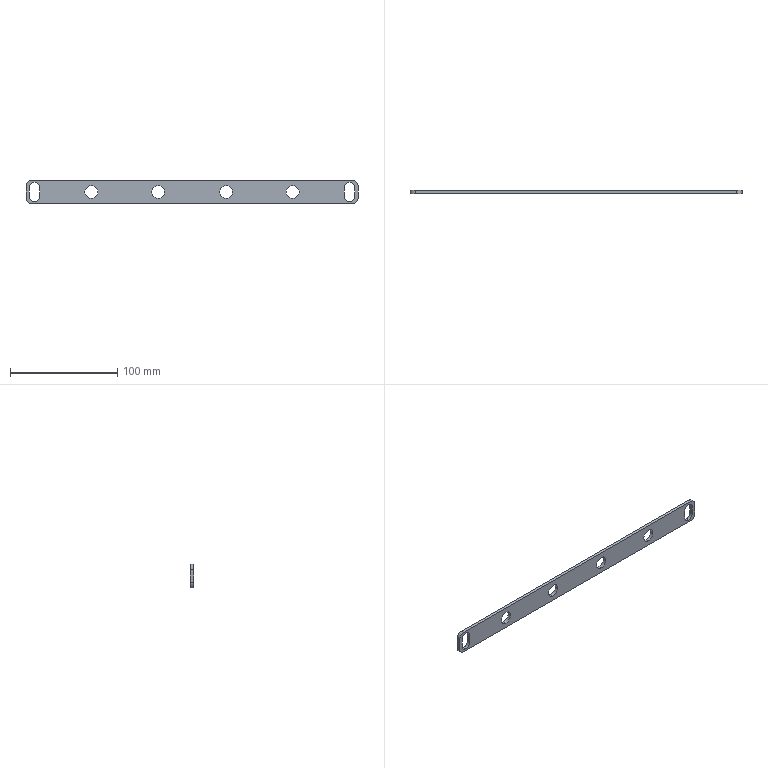Part | 1 solid | 28 faces | box 310 x 3 x 22 mm | volume 18087 mm3 | cylinder 18 | plane 10 | commonest cylinder face diameters 10 x10 12 x8
STEP:
#1=CARTESIAN_POINT('',(152.,3.,-4.));
#2=VERTEX_POINT('',#1);
#3=CARTESIAN_POINT('',(147.,3.,-9.));
#4=VERTEX_POINT('',#3);
#5=CARTESIAN_POINT('',(147.,3.,-4.));
#6=DIRECTION('',(0.,1.,0.));
#7=DIRECTION('',(0.,0.,-1.));
#8=AXIS2_PLACEMENT_3D('',#5,#6,#7);
#9=CIRCLE('',#8,5.);
#10=EDGE_CURVE('',#2,#4,#9,.T.);
#11=ORIENTED_EDGE('',*,*,#10,.T.);
#12=CARTESIAN_POINT('',(147.,0.,-9.));
#13=VERTEX_POINT('',#12);
#14=CARTESIAN_POINT('',(147.,3.,-9.));
#15=DIRECTION('',(0.,-1.,0.));
#16=VECTOR('',#15,1000.);
#17=LINE('',#14,#16);
#18=EDGE_CURVE('',#4,#13,#17,.T.);
#19=ORIENTED_EDGE('',*,*,#18,.T.);
#20=CARTESIAN_POINT('',(152.,0.,-4.));
#21=VERTEX_POINT('',#20);
#22=CARTESIAN_POINT('',(147.,0.,-4.));
#23=DIRECTION('',(0.,1.,0.));
#24=DIRECTION('',(0.,0.,-1.));
#25=AXIS2_PLACEMENT_3D('',#22,#23,#24);
#26=CIRCLE('',#25,5.);
#27=EDGE_CURVE('',#21,#13,#26,.T.);
#28=ORIENTED_EDGE('',*,*,#27,.F.);
#29=CARTESIAN_POINT('',(152.,3.,-4.));
#30=DIRECTION('',(0.,-1.,0.));
#31=VECTOR('',#30,1000.);
#32=LINE('',#29,#31);
#33=EDGE_CURVE('',#2,#21,#32,.T.);
#34=ORIENTED_EDGE('',*,*,#33,.F.);
#35=EDGE_LOOP('',(#11,#19,#28,#34));
#36=FACE_OUTER_BOUND('',#35,.T.);
#37=CARTESIAN_POINT('',(147.,3.,-4.));
#38=DIRECTION('',(0.,-1.,0.));
#39=DIRECTION('',(0.,0.,-1.));
#40=AXIS2_PLACEMENT_3D('',#37,#38,#39);
#41=CYLINDRICAL_SURFACE('',#40,5.);
#42=ADVANCED_FACE('',(#36),#41,.F.);
#43=CARTESIAN_POINT('',(94.,3.,-6.));
#44=VERTEX_POINT('',#43);
#45=CARTESIAN_POINT('',(94.,3.,6.));
#46=VERTEX_POINT('',#45);
#47=CARTESIAN_POINT('',(94.,3.,0.));
#48=DIRECTION('',(0.,1.,0.));
#49=DIRECTION('',(0.,0.,1.));
#50=AXIS2_PLACEMENT_3D('',#47,#48,#49);
#51=CIRCLE('',#50,6.);
#52=EDGE_CURVE('',#44,#46,#51,.T.);
#53=ORIENTED_EDGE('',*,*,#52,.T.);
#54=CARTESIAN_POINT('',(94.,0.,6.));
#55=VERTEX_POINT('',#54);
#56=CARTESIAN_POINT('',(94.,3.,6.));
#57=DIRECTION('',(0.,-1.,0.));
#58=VECTOR('',#57,1000.);
#59=LINE('',#56,#58);
#60=EDGE_CURVE('',#46,#55,#59,.T.);
#61=ORIENTED_EDGE('',*,*,#60,.T.);
#62=CARTESIAN_POINT('',(94.,0.,-6.));
#63=VERTEX_POINT('',#62);
#64=CARTESIAN_POINT('',(94.,0.,0.));
#65=DIRECTION('',(0.,1.,0.));
#66=DIRECTION('',(0.,0.,1.));
#67=AXIS2_PLACEMENT_3D('',#64,#65,#66);
#68=CIRCLE('',#67,6.);
#69=EDGE_CURVE('',#63,#55,#68,.T.);
#70=ORIENTED_EDGE('',*,*,#69,.F.);
#71=CARTESIAN_POINT('',(94.,3.,-6.));
#72=DIRECTION('',(0.,-1.,0.));
#73=VECTOR('',#72,1000.);
#74=LINE('',#71,#73);
#75=EDGE_CURVE('',#44,#63,#74,.T.);
#76=ORIENTED_EDGE('',*,*,#75,.F.);
#77=EDGE_LOOP('',(#53,#61,#70,#76));
#78=FACE_OUTER_BOUND('',#77,.T.);
#79=CARTESIAN_POINT('',(94.,3.,0.));
#80=DIRECTION('',(0.,-1.,0.));
#81=DIRECTION('',(0.,0.,-1.));
#82=AXIS2_PLACEMENT_3D('',#79,#80,#81);
#83=CYLINDRICAL_SURFACE('',#82,6.);
#84=ADVANCED_FACE('',(#78),#83,.F.);
#85=CARTESIAN_POINT('',(31.8,3.,-6.));
#86=VERTEX_POINT('',#85);
#87=CARTESIAN_POINT('',(31.8,3.,6.));
#88=VERTEX_POINT('',#87);
#89=CARTESIAN_POINT('',(31.8,3.,0.));
#90=DIRECTION('',(0.,1.,0.));
#91=DIRECTION('',(0.,0.,1.));
#92=AXIS2_PLACEMENT_3D('',#89,#90,#91);
#93=CIRCLE('',#92,6.);
#94=EDGE_CURVE('',#86,#88,#93,.T.);
#95=ORIENTED_EDGE('',*,*,#94,.T.);
#96=CARTESIAN_POINT('',(31.8,0.,6.));
#97=VERTEX_POINT('',#96);
#98=CARTESIAN_POINT('',(31.8,3.,6.));
#99=DIRECTION('',(0.,-1.,0.));
#100=VECTOR('',#99,1000.);
#101=LINE('',#98,#100);
#102=EDGE_CURVE('',#88,#97,#101,.T.);
#103=ORIENTED_EDGE('',*,*,#102,.T.);
#104=CARTESIAN_POINT('',(31.8,0.,-6.));
#105=VERTEX_POINT('',#104);
#106=CARTESIAN_POINT('',(31.8,0.,0.));
#107=DIRECTION('',(0.,1.,0.));
#108=DIRECTION('',(0.,0.,1.));
#109=AXIS2_PLACEMENT_3D('',#106,#107,#108);
#110=CIRCLE('',#109,6.);
#111=EDGE_CURVE('',#105,#97,#110,.T.);
#112=ORIENTED_EDGE('',*,*,#111,.F.);
#113=CARTESIAN_POINT('',(31.8,3.,-6.));
#114=DIRECTION('',(0.,-1.,0.));
#115=VECTOR('',#114,1000.);
#116=LINE('',#113,#115);
#117=EDGE_CURVE('',#86,#105,#116,.T.);
#118=ORIENTED_EDGE('',*,*,#117,.F.);
#119=EDGE_LOOP('',(#95,#103,#112,#118));
#120=FACE_OUTER_BOUND('',#119,.T.);
#121=CARTESIAN_POINT('',(31.8,3.,0.));
#122=DIRECTION('',(0.,-1.,0.));
#123=DIRECTION('',(0.,0.,-1.));
#124=AXIS2_PLACEMENT_3D('',#121,#122,#123);
#125=CYLINDRICAL_SURFACE('',#124,6.);
#126=ADVANCED_FACE('',(#120),#125,.F.);
#127=CARTESIAN_POINT('',(-31.7,3.,-6.));
#128=VERTEX_POINT('',#127);
#129=CARTESIAN_POINT('',(-31.7,3.,6.));
#130=VERTEX_POINT('',#129);
#131=CARTESIAN_POINT('',(-31.7,3.,0.));
#132=DIRECTION('',(0.,1.,0.));
#133=DIRECTION('',(0.,0.,1.));
#134=AXIS2_PLACEMENT_3D('',#131,#132,#133);
#135=CIRCLE('',#134,6.);
#136=EDGE_CURVE('',#128,#130,#135,.T.);
#137=ORIENTED_EDGE('',*,*,#136,.T.);
#138=CARTESIAN_POINT('',(-31.7,0.,6.));
#139=VERTEX_POINT('',#138);
#140=CARTESIAN_POINT('',(-31.7,3.,6.));
#141=DIRECTION('',(0.,-1.,0.));
#142=VECTOR('',#141,1000.);
#143=LINE('',#140,#142);
#144=EDGE_CURVE('',#130,#139,#143,.T.);
#145=ORIENTED_EDGE('',*,*,#144,.T.);
#146=CARTESIAN_POINT('',(-31.7,0.,-6.));
#147=VERTEX_POINT('',#146);
#148=CARTESIAN_POINT('',(-31.7,0.,0.));
#149=DIRECTION('',(0.,1.,0.));
#150=DIRECTION('',(0.,0.,1.));
#151=AXIS2_PLACEMENT_3D('',#148,#149,#150);
#152=CIRCLE('',#151,6.);
#153=EDGE_CURVE('',#147,#139,#152,.T.);
#154=ORIENTED_EDGE('',*,*,#153,.F.);
#155=CARTESIAN_POINT('',(-31.7,3.,-6.));
#156=DIRECTION('',(0.,-1.,0.));
#157=VECTOR('',#156,1000.);
#158=LINE('',#155,#157);
#159=EDGE_CURVE('',#128,#147,#158,.T.);
#160=ORIENTED_EDGE('',*,*,#159,.F.);
#161=EDGE_LOOP('',(#137,#145,#154,#160));
#162=FACE_OUTER_BOUND('',#161,.T.);
#163=CARTESIAN_POINT('',(-31.7,3.,0.));
#164=DIRECTION('',(0.,-1.,0.));
#165=DIRECTION('',(0.,0.,-1.));
#166=AXIS2_PLACEMENT_3D('',#163,#164,#165);
#167=CYLINDRICAL_SURFACE('',#166,6.);
#168=ADVANCED_FACE('',(#162),#167,.F.);
#169=CARTESIAN_POINT('',(-94.,3.,-6.));
#170=VERTEX_POINT('',#169);
#171=CARTESIAN_POINT('',(-94.,3.,6.));
#172=VERTEX_POINT('',#171);
#173=CARTESIAN_POINT('',(-94.,3.,0.));
#174=DIRECTION('',(0.,1.,0.));
#175=DIRECTION('',(0.,0.,1.));
#176=AXIS2_PLACEMENT_3D('',#173,#174,#175);
#177=CIRCLE('',#176,6.);
#178=EDGE_CURVE('',#170,#172,#177,.T.);
#179=ORIENTED_EDGE('',*,*,#178,.T.);
#180=CARTESIAN_POINT('',(-94.,0.,6.));
#181=VERTEX_POINT('',#180);
#182=CARTESIAN_POINT('',(-94.,3.,6.));
#183=DIRECTION('',(0.,-1.,0.));
#184=VECTOR('',#183,1000.);
#185=LINE('',#182,#184);
#186=EDGE_CURVE('',#172,#181,#185,.T.);
#187=ORIENTED_EDGE('',*,*,#186,.T.);
#188=CARTESIAN_POINT('',(-94.,0.,-6.));
#189=VERTEX_POINT('',#188);
#190=CARTESIAN_POINT('',(-94.,0.,0.));
#191=DIRECTION('',(0.,1.,0.));
#192=DIRECTION('',(0.,0.,1.));
#193=AXIS2_PLACEMENT_3D('',#190,#191,#192);
#194=CIRCLE('',#193,6.);
#195=EDGE_CURVE('',#189,#181,#194,.T.);
#196=ORIENTED_EDGE('',*,*,#195,.F.);
#197=CARTESIAN_POINT('',(-94.,3.,-6.));
#198=DIRECTION('',(0.,-1.,0.));
#199=VECTOR('',#198,1000.);
#200=LINE('',#197,#199);
#201=EDGE_CURVE('',#170,#189,#200,.T.);
#202=ORIENTED_EDGE('',*,*,#201,.F.);
#203=EDGE_LOOP('',(#179,#187,#196,#202));
#204=FACE_OUTER_BOUND('',#203,.T.);
#205=CARTESIAN_POINT('',(-94.,3.,0.));
#206=DIRECTION('',(0.,-1.,0.));
#207=DIRECTION('',(0.,0.,-1.));
#208=AXIS2_PLACEMENT_3D('',#205,#206,#207);
#209=CYLINDRICAL_SURFACE('',#208,6.);
#210=ADVANCED_FACE('',(#204),#209,.F.);
#211=CARTESIAN_POINT('',(-142.,3.,-4.));
#212=VERTEX_POINT('',#211);
#213=CARTESIAN_POINT('',(-147.,3.,-9.));
#214=VERTEX_POINT('',#213);
#215=CARTESIAN_POINT('',(-147.,3.,-4.));
#216=DIRECTION('',(0.,1.,0.));
#217=DIRECTION('',(0.,0.,1.));
#218=AXIS2_PLACEMENT_3D('',#215,#216,#217);
#219=CIRCLE('',#218,5.);
#220=EDGE_CURVE('',#212,#214,#219,.T.);
#221=ORIENTED_EDGE('',*,*,#220,.T.);
#222=CARTESIAN_POINT('',(-147.,0.,-9.));
#223=VERTEX_POINT('',#222);
#224=CARTESIAN_POINT('',(-147.,3.,-9.));
#225=DIRECTION('',(0.,-1.,0.));
#226=VECTOR('',#225,1000.);
#227=LINE('',#224,#226);
#228=EDGE_CURVE('',#214,#223,#227,.T.);
#229=ORIENTED_EDGE('',*,*,#228,.T.);
#230=CARTESIAN_POINT('',(-142.,0.,-4.));
#231=VERTEX_POINT('',#230);
#232=CARTESIAN_POINT('',(-147.,0.,-4.));
#233=DIRECTION('',(0.,1.,0.));
#234=DIRECTION('',(0.,0.,1.));
#235=AXIS2_PLACEMENT_3D('',#232,#233,#234);
#236=CIRCLE('',#235,5.);
#237=EDGE_CURVE('',#231,#223,#236,.T.);
#238=ORIENTED_EDGE('',*,*,#237,.F.);
#239=CARTESIAN_POINT('',(-142.,3.,-4.));
#240=DIRECTION('',(0.,-1.,0.));
#241=VECTOR('',#240,1000.);
#242=LINE('',#239,#241);
#243=EDGE_CURVE('',#212,#231,#242,.T.);
#244=ORIENTED_EDGE('',*,*,#243,.F.);
#245=EDGE_LOOP('',(#221,#229,#238,#244));
#246=FACE_OUTER_BOUND('',#245,.T.);
#247=CARTESIAN_POINT('',(-147.,3.,-4.));
#248=DIRECTION('',(0.,-1.,0.));
#249=DIRECTION('',(0.,0.,-1.));
#250=AXIS2_PLACEMENT_3D('',#247,#248,#249);
#251=CYLINDRICAL_SURFACE('',#250,5.);
#252=ADVANCED_FACE('',(#246),#251,.F.);
#253=ORIENTED_EDGE('',*,*,#94,.F.);
#254=CARTESIAN_POINT('',(31.8,3.,0.));
#255=DIRECTION('',(0.,1.,0.));
#256=DIRECTION('',(0.,0.,1.));
#257=AXIS2_PLACEMENT_3D('',#254,#255,#256);
#258=CIRCLE('',#257,6.);
#259=EDGE_CURVE('',#88,#86,#258,.T.);
#260=ORIENTED_EDGE('',*,*,#259,.F.);
#261=EDGE_LOOP('',(#253,#260));
#262=FACE_BOUND('',#261,.T.);
#263=ORIENTED_EDGE('',*,*,#178,.F.);
#264=CARTESIAN_POINT('',(-94.,3.,0.));
#265=DIRECTION('',(0.,1.,0.));
#266=DIRECTION('',(0.,0.,1.));
#267=AXIS2_PLACEMENT_3D('',#264,#265,#266);
#268=CIRCLE('',#267,6.);
#269=EDGE_CURVE('',#172,#170,#268,.T.);
#270=ORIENTED_EDGE('',*,*,#269,.F.);
#271=EDGE_LOOP('',(#263,#270));
#272=FACE_BOUND('',#271,.T.);
#273=CARTESIAN_POINT('',(-150.,3.,11.));
#274=VERTEX_POINT('',#273);
#275=CARTESIAN_POINT('',(150.,3.,11.));
#276=VERTEX_POINT('',#275);
#277=CARTESIAN_POINT('',(-155.,3.,11.));
#278=DIRECTION('',(1.,0.,0.));
#279=VECTOR('',#278,1000.);
#280=LINE('',#277,#279);
#281=EDGE_CURVE('',#274,#276,#280,.T.);
#282=ORIENTED_EDGE('',*,*,#281,.T.);
#283=CARTESIAN_POINT('',(155.,3.,6.));
#284=VERTEX_POINT('',#283);
#285=CARTESIAN_POINT('',(150.,3.,6.));
#286=DIRECTION('',(0.,1.,0.));
#287=DIRECTION('',(0.,0.,1.));
#288=AXIS2_PLACEMENT_3D('',#285,#286,#287);
#289=CIRCLE('',#288,5.);
#290=EDGE_CURVE('',#276,#284,#289,.T.);
#291=ORIENTED_EDGE('',*,*,#290,.T.);
#292=CARTESIAN_POINT('',(155.,3.,-6.));
#293=VERTEX_POINT('',#292);
#294=CARTESIAN_POINT('',(155.,3.,-11.));
#295=DIRECTION('',(0.,0.,-1.));
#296=VECTOR('',#295,1000.);
#297=LINE('',#294,#296);
#298=EDGE_CURVE('',#284,#293,#297,.T.);
#299=ORIENTED_EDGE('',*,*,#298,.T.);
#300=CARTESIAN_POINT('',(150.,3.,-11.));
#301=VERTEX_POINT('',#300);
#302=CARTESIAN_POINT('',(150.,3.,-6.));
#303=DIRECTION('',(0.,1.,0.));
#304=DIRECTION('',(0.,0.,1.));
#305=AXIS2_PLACEMENT_3D('',#302,#303,#304);
#306=CIRCLE('',#305,5.);
#307=EDGE_CURVE('',#293,#301,#306,.T.);
#308=ORIENTED_EDGE('',*,*,#307,.T.);
#309=CARTESIAN_POINT('',(-150.,3.,-11.));
#310=VERTEX_POINT('',#309);
#311=CARTESIAN_POINT('',(-155.,3.,-11.));
#312=DIRECTION('',(-1.,0.,0.));
#313=VECTOR('',#312,1000.);
#314=LINE('',#311,#313);
#315=EDGE_CURVE('',#301,#310,#314,.T.);
#316=ORIENTED_EDGE('',*,*,#315,.T.);
#317=CARTESIAN_POINT('',(-155.,3.,-6.));
#318=VERTEX_POINT('',#317);
#319=CARTESIAN_POINT('',(-150.,3.,-6.));
#320=DIRECTION('',(0.,1.,0.));
#321=DIRECTION('',(0.,0.,1.));
#322=AXIS2_PLACEMENT_3D('',#319,#320,#321);
#323=CIRCLE('',#322,5.);
#324=EDGE_CURVE('',#310,#318,#323,.T.);
#325=ORIENTED_EDGE('',*,*,#324,.T.);
#326=CARTESIAN_POINT('',(-155.,3.,6.));
#327=VERTEX_POINT('',#326);
#328=CARTESIAN_POINT('',(-155.,3.,-11.));
#329=DIRECTION('',(0.,0.,1.));
#330=VECTOR('',#329,1000.);
#331=LINE('',#328,#330);
#332=EDGE_CURVE('',#318,#327,#331,.T.);
#333=ORIENTED_EDGE('',*,*,#332,.T.);
#334=CARTESIAN_POINT('',(-150.,3.,6.));
#335=DIRECTION('',(0.,1.,0.));
#336=DIRECTION('',(0.,0.,1.));
#337=AXIS2_PLACEMENT_3D('',#334,#335,#336);
#338=CIRCLE('',#337,5.);
#339=EDGE_CURVE('',#327,#274,#338,.T.);
#340=ORIENTED_EDGE('',*,*,#339,.T.);
#341=EDGE_LOOP('',(#282,#291,#299,#308,#316,#325,#333,#340));
#342=FACE_OUTER_BOUND('',#341,.T.);
#343=CARTESIAN_POINT('',(-142.,3.,4.));
#344=VERTEX_POINT('',#343);
#345=CARTESIAN_POINT('',(-142.,3.,4.));
#346=DIRECTION('',(0.,0.,-1.));
#347=VECTOR('',#346,1000.);
#348=LINE('',#345,#347);
#349=EDGE_CURVE('',#344,#212,#348,.T.);
#350=ORIENTED_EDGE('',*,*,#349,.F.);
#351=CARTESIAN_POINT('',(-152.,3.,4.));
#352=VERTEX_POINT('',#351);
#353=CARTESIAN_POINT('',(-147.,3.,4.));
#354=DIRECTION('',(0.,1.,0.));
#355=DIRECTION('',(0.,0.,1.));
#356=AXIS2_PLACEMENT_3D('',#353,#354,#355);
#357=CIRCLE('',#356,5.);
#358=EDGE_CURVE('',#352,#344,#357,.T.);
#359=ORIENTED_EDGE('',*,*,#358,.F.);
#360=CARTESIAN_POINT('',(-152.,3.,-4.));
#361=VERTEX_POINT('',#360);
#362=CARTESIAN_POINT('',(-152.,3.,4.));
#363=DIRECTION('',(0.,0.,1.));
#364=VECTOR('',#363,1000.);
#365=LINE('',#362,#364);
#366=EDGE_CURVE('',#361,#352,#365,.T.);
#367=ORIENTED_EDGE('',*,*,#366,.F.);
#368=CARTESIAN_POINT('',(-147.,3.,-4.));
#369=DIRECTION('',(0.,1.,0.));
#370=DIRECTION('',(0.,0.,1.));
#371=AXIS2_PLACEMENT_3D('',#368,#369,#370);
#372=CIRCLE('',#371,5.);
#373=EDGE_CURVE('',#214,#361,#372,.T.);
#374=ORIENTED_EDGE('',*,*,#373,.F.);
#375=ORIENTED_EDGE('',*,*,#220,.F.);
#376=EDGE_LOOP('',(#350,#359,#367,#374,#375));
#377=FACE_BOUND('',#376,.T.);
#378=ORIENTED_EDGE('',*,*,#136,.F.);
#379=CARTESIAN_POINT('',(-31.7,3.,0.));
#380=DIRECTION('',(0.,1.,0.));
#381=DIRECTION('',(0.,0.,1.));
#382=AXIS2_PLACEMENT_3D('',#379,#380,#381);
#383=CIRCLE('',#382,6.);
#384=EDGE_CURVE('',#130,#128,#383,.T.);
#385=ORIENTED_EDGE('',*,*,#384,.F.);
#386=EDGE_LOOP('',(#378,#385));
#387=FACE_BOUND('',#386,.T.);
#388=ORIENTED_EDGE('',*,*,#52,.F.);
#389=CARTESIAN_POINT('',(94.,3.,0.));
#390=DIRECTION('',(0.,1.,0.));
#391=DIRECTION('',(0.,0.,1.));
#392=AXIS2_PLACEMENT_3D('',#389,#390,#391);
#393=CIRCLE('',#392,6.);
#394=EDGE_CURVE('',#46,#44,#393,.T.);
#395=ORIENTED_EDGE('',*,*,#394,.F.);
#396=EDGE_LOOP('',(#388,#395));
#397=FACE_BOUND('',#396,.T.);
#398=CARTESIAN_POINT('',(152.,3.,4.));
#399=VERTEX_POINT('',#398);
#400=CARTESIAN_POINT('',(152.,3.,4.));
#401=DIRECTION('',(0.,0.,-1.));
#402=VECTOR('',#401,1000.);
#403=LINE('',#400,#402);
#404=EDGE_CURVE('',#399,#2,#403,.T.);
#405=ORIENTED_EDGE('',*,*,#404,.F.);
#406=CARTESIAN_POINT('',(142.,3.,4.));
#407=VERTEX_POINT('',#406);
#408=CARTESIAN_POINT('',(147.,3.,4.));
#409=DIRECTION('',(0.,1.,0.));
#410=DIRECTION('',(0.,0.,-1.));
#411=AXIS2_PLACEMENT_3D('',#408,#409,#410);
#412=CIRCLE('',#411,5.);
#413=EDGE_CURVE('',#407,#399,#412,.T.);
#414=ORIENTED_EDGE('',*,*,#413,.F.);
#415=CARTESIAN_POINT('',(142.,3.,-4.));
#416=VERTEX_POINT('',#415);
#417=CARTESIAN_POINT('',(142.,3.,4.));
#418=DIRECTION('',(0.,0.,1.));
#419=VECTOR('',#418,1000.);
#420=LINE('',#417,#419);
#421=EDGE_CURVE('',#416,#407,#420,.T.);
#422=ORIENTED_EDGE('',*,*,#421,.F.);
#423=CARTESIAN_POINT('',(147.,3.,-4.));
#424=DIRECTION('',(0.,1.,0.));
#425=DIRECTION('',(0.,0.,-1.));
#426=AXIS2_PLACEMENT_3D('',#423,#424,#425);
#427=CIRCLE('',#426,5.);
#428=EDGE_CURVE('',#4,#416,#427,.T.);
#429=ORIENTED_EDGE('',*,*,#428,.F.);
#430=ORIENTED_EDGE('',*,*,#10,.F.);
#431=EDGE_LOOP('',(#405,#414,#422,#429,#430));
#432=FACE_BOUND('',#431,.T.);
#433=CARTESIAN_POINT('',(0.,3.,0.));
#434=DIRECTION('',(0.,1.,0.));
#435=DIRECTION('',(0.,0.,1.));
#436=AXIS2_PLACEMENT_3D('',#433,#434,#435);
#437=PLANE('',#436);
#438=ADVANCED_FACE('',(#262,#272,#342,#377,#387,#397,#432),#437,.T.);
#439=ORIENTED_EDGE('',*,*,#69,.T.);
#440=CARTESIAN_POINT('',(94.,0.,0.));
#441=DIRECTION('',(0.,1.,0.));
#442=DIRECTION('',(0.,0.,1.));
#443=AXIS2_PLACEMENT_3D('',#440,#441,#442);
#444=CIRCLE('',#443,6.);
#445=EDGE_CURVE('',#55,#63,#444,.T.);
#446=ORIENTED_EDGE('',*,*,#445,.T.);
#447=EDGE_LOOP('',(#439,#446));
#448=FACE_BOUND('',#447,.T.);
#449=ORIENTED_EDGE('',*,*,#111,.T.);
#450=CARTESIAN_POINT('',(31.8,0.,0.));
#451=DIRECTION('',(0.,1.,0.));
#452=DIRECTION('',(0.,0.,1.));
#453=AXIS2_PLACEMENT_3D('',#450,#451,#452);
#454=CIRCLE('',#453,6.);
#455=EDGE_CURVE('',#97,#105,#454,.T.);
#456=ORIENTED_EDGE('',*,*,#455,.T.);
#457=EDGE_LOOP('',(#449,#456));
#458=FACE_BOUND('',#457,.T.);
#459=ORIENTED_EDGE('',*,*,#153,.T.);
#460=CARTESIAN_POINT('',(-31.7,0.,0.));
#461=DIRECTION('',(0.,1.,0.));
#462=DIRECTION('',(0.,0.,1.));
#463=AXIS2_PLACEMENT_3D('',#460,#461,#462);
#464=CIRCLE('',#463,6.);
#465=EDGE_CURVE('',#139,#147,#464,.T.);
#466=ORIENTED_EDGE('',*,*,#465,.T.);
#467=EDGE_LOOP('',(#459,#466));
#468=FACE_BOUND('',#467,.T.);
#469=ORIENTED_EDGE('',*,*,#195,.T.);
#470=CARTESIAN_POINT('',(-94.,0.,0.));
#471=DIRECTION('',(0.,1.,0.));
#472=DIRECTION('',(0.,0.,1.));
#473=AXIS2_PLACEMENT_3D('',#470,#471,#472);
#474=CIRCLE('',#473,6.);
#475=EDGE_CURVE('',#181,#189,#474,.T.);
#476=ORIENTED_EDGE('',*,*,#475,.T.);
#477=EDGE_LOOP('',(#469,#476));
#478=FACE_BOUND('',#477,.T.);
#479=CARTESIAN_POINT('',(-152.,0.,4.));
#480=VERTEX_POINT('',#479);
#481=CARTESIAN_POINT('',(-142.,0.,4.));
#482=VERTEX_POINT('',#481);
#483=CARTESIAN_POINT('',(-147.,0.,4.));
#484=DIRECTION('',(0.,1.,0.));
#485=DIRECTION('',(0.,0.,1.));
#486=AXIS2_PLACEMENT_3D('',#483,#484,#485);
#487=CIRCLE('',#486,5.);
#488=EDGE_CURVE('',#480,#482,#487,.T.);
#489=ORIENTED_EDGE('',*,*,#488,.T.);
#490=CARTESIAN_POINT('',(-142.,0.,4.));
#491=DIRECTION('',(0.,0.,-1.));
#492=VECTOR('',#491,1000.);
#493=LINE('',#490,#492);
#494=EDGE_CURVE('',#482,#231,#493,.T.);
#495=ORIENTED_EDGE('',*,*,#494,.T.);
#496=ORIENTED_EDGE('',*,*,#237,.T.);
#497=CARTESIAN_POINT('',(-152.,0.,-4.));
#498=VERTEX_POINT('',#497);
#499=CARTESIAN_POINT('',(-147.,0.,-4.));
#500=DIRECTION('',(0.,1.,0.));
#501=DIRECTION('',(0.,0.,1.));
#502=AXIS2_PLACEMENT_3D('',#499,#500,#501);
#503=CIRCLE('',#502,5.);
#504=EDGE_CURVE('',#223,#498,#503,.T.);
#505=ORIENTED_EDGE('',*,*,#504,.T.);
#506=CARTESIAN_POINT('',(-152.,0.,4.));
#507=DIRECTION('',(0.,0.,1.));
#508=VECTOR('',#507,1000.);
#509=LINE('',#506,#508);
#510=EDGE_CURVE('',#498,#480,#509,.T.);
#511=ORIENTED_EDGE('',*,*,#510,.T.);
#512=EDGE_LOOP('',(#489,#495,#496,#505,#511));
#513=FACE_BOUND('',#512,.T.);
#514=CARTESIAN_POINT('',(155.,0.,6.));
#515=VERTEX_POINT('',#514);
#516=CARTESIAN_POINT('',(155.,0.,-6.));
#517=VERTEX_POINT('',#516);
#518=CARTESIAN_POINT('',(155.,0.,-11.));
#519=DIRECTION('',(0.,0.,-1.));
#520=VECTOR('',#519,1000.);
#521=LINE('',#518,#520);
#522=EDGE_CURVE('',#515,#517,#521,.T.);
#523=ORIENTED_EDGE('',*,*,#522,.F.);
#524=CARTESIAN_POINT('',(150.,0.,11.));
#525=VERTEX_POINT('',#524);
#526=CARTESIAN_POINT('',(150.,0.,6.));
#527=DIRECTION('',(0.,-1.,0.));
#528=DIRECTION('',(0.,0.,1.));
#529=AXIS2_PLACEMENT_3D('',#526,#527,#528);
#530=CIRCLE('',#529,5.);
#531=EDGE_CURVE('',#515,#525,#530,.T.);
#532=ORIENTED_EDGE('',*,*,#531,.T.);
#533=CARTESIAN_POINT('',(-150.,0.,11.));
#534=VERTEX_POINT('',#533);
#535=CARTESIAN_POINT('',(-155.,0.,11.));
#536=DIRECTION('',(1.,0.,0.));
#537=VECTOR('',#536,1000.);
#538=LINE('',#535,#537);
#539=EDGE_CURVE('',#534,#525,#538,.T.);
#540=ORIENTED_EDGE('',*,*,#539,.F.);
#541=CARTESIAN_POINT('',(-155.,0.,6.));
#542=VERTEX_POINT('',#541);
#543=CARTESIAN_POINT('',(-150.,0.,6.));
#544=DIRECTION('',(0.,-1.,0.));
#545=DIRECTION('',(0.,0.,1.));
#546=AXIS2_PLACEMENT_3D('',#543,#544,#545);
#547=CIRCLE('',#546,5.);
#548=EDGE_CURVE('',#534,#542,#547,.T.);
#549=ORIENTED_EDGE('',*,*,#548,.T.);
#550=CARTESIAN_POINT('',(-155.,0.,-6.));
#551=VERTEX_POINT('',#550);
#552=CARTESIAN_POINT('',(-155.,0.,-11.));
#553=DIRECTION('',(0.,0.,1.));
#554=VECTOR('',#553,1000.);
#555=LINE('',#552,#554);
#556=EDGE_CURVE('',#551,#542,#555,.T.);
#557=ORIENTED_EDGE('',*,*,#556,.F.);
#558=CARTESIAN_POINT('',(-150.,0.,-11.));
#559=VERTEX_POINT('',#558);
#560=CARTESIAN_POINT('',(-150.,0.,-6.));
#561=DIRECTION('',(0.,-1.,0.));
#562=DIRECTION('',(0.,0.,1.));
#563=AXIS2_PLACEMENT_3D('',#560,#561,#562);
#564=CIRCLE('',#563,5.);
#565=EDGE_CURVE('',#551,#559,#564,.T.);
#566=ORIENTED_EDGE('',*,*,#565,.T.);
#567=CARTESIAN_POINT('',(150.,0.,-11.));
#568=VERTEX_POINT('',#567);
#569=CARTESIAN_POINT('',(-155.,0.,-11.));
#570=DIRECTION('',(-1.,0.,0.));
#571=VECTOR('',#570,1000.);
#572=LINE('',#569,#571);
#573=EDGE_CURVE('',#568,#559,#572,.T.);
#574=ORIENTED_EDGE('',*,*,#573,.F.);
#575=CARTESIAN_POINT('',(150.,0.,-6.));
#576=DIRECTION('',(0.,-1.,0.));
#577=DIRECTION('',(0.,0.,1.));
#578=AXIS2_PLACEMENT_3D('',#575,#576,#577);
#579=CIRCLE('',#578,5.);
#580=EDGE_CURVE('',#568,#517,#579,.T.);
#581=ORIENTED_EDGE('',*,*,#580,.T.);
#582=EDGE_LOOP('',(#523,#532,#540,#549,#557,#566,#574,#581));
#583=FACE_OUTER_BOUND('',#582,.T.);
#584=CARTESIAN_POINT('',(142.,0.,4.));
#585=VERTEX_POINT('',#584);
#586=CARTESIAN_POINT('',(152.,0.,4.));
#587=VERTEX_POINT('',#586);
#588=CARTESIAN_POINT('',(147.,0.,4.));
#589=DIRECTION('',(0.,1.,0.));
#590=DIRECTION('',(0.,0.,-1.));
#591=AXIS2_PLACEMENT_3D('',#588,#589,#590);
#592=CIRCLE('',#591,5.);
#593=EDGE_CURVE('',#585,#587,#592,.T.);
#594=ORIENTED_EDGE('',*,*,#593,.T.);
#595=CARTESIAN_POINT('',(152.,0.,4.));
#596=DIRECTION('',(0.,0.,-1.));
#597=VECTOR('',#596,1000.);
#598=LINE('',#595,#597);
#599=EDGE_CURVE('',#587,#21,#598,.T.);
#600=ORIENTED_EDGE('',*,*,#599,.T.);
#601=ORIENTED_EDGE('',*,*,#27,.T.);
#602=CARTESIAN_POINT('',(142.,0.,-4.));
#603=VERTEX_POINT('',#602);
#604=CARTESIAN_POINT('',(147.,0.,-4.));
#605=DIRECTION('',(0.,1.,0.));
#606=DIRECTION('',(0.,0.,-1.));
#607=AXIS2_PLACEMENT_3D('',#604,#605,#606);
#608=CIRCLE('',#607,5.);
#609=EDGE_CURVE('',#13,#603,#608,.T.);
#610=ORIENTED_EDGE('',*,*,#609,.T.);
#611=CARTESIAN_POINT('',(142.,0.,4.));
#612=DIRECTION('',(0.,0.,1.));
#613=VECTOR('',#612,1000.);
#614=LINE('',#611,#613);
#615=EDGE_CURVE('',#603,#585,#614,.T.);
#616=ORIENTED_EDGE('',*,*,#615,.T.);
#617=EDGE_LOOP('',(#594,#600,#601,#610,#616));
#618=FACE_BOUND('',#617,.T.);
#619=CARTESIAN_POINT('',(0.,0.,0.));
#620=DIRECTION('',(0.,1.,0.));
#621=DIRECTION('',(0.,0.,1.));
#622=AXIS2_PLACEMENT_3D('',#619,#620,#621);
#623=PLANE('',#622);
#624=ADVANCED_FACE('',(#448,#458,#468,#478,#513,#583,#618),#623,.F.);
#625=ORIENTED_EDGE('',*,*,#298,.F.);
#626=CARTESIAN_POINT('',(155.,3.,6.));
#627=DIRECTION('',(0.,-1.,0.));
#628=VECTOR('',#627,1000.);
#629=LINE('',#626,#628);
#630=EDGE_CURVE('',#284,#515,#629,.T.);
#631=ORIENTED_EDGE('',*,*,#630,.T.);
#632=ORIENTED_EDGE('',*,*,#522,.T.);
#633=CARTESIAN_POINT('',(155.,3.,-6.));
#634=DIRECTION('',(0.,1.,0.));
#635=VECTOR('',#634,1000.);
#636=LINE('',#633,#635);
#637=EDGE_CURVE('',#517,#293,#636,.T.);
#638=ORIENTED_EDGE('',*,*,#637,.T.);
#639=EDGE_LOOP('',(#625,#631,#632,#638));
#640=FACE_OUTER_BOUND('',#639,.T.);
#641=CARTESIAN_POINT('',(155.,3.,-11.));
#642=DIRECTION('',(-1.,0.,0.));
#643=DIRECTION('',(0.,0.,1.));
#644=AXIS2_PLACEMENT_3D('',#641,#642,#643);
#645=PLANE('',#644);
#646=ADVANCED_FACE('',(#640),#645,.F.);
#647=ORIENTED_EDGE('',*,*,#573,.T.);
#648=CARTESIAN_POINT('',(-150.,3.,-11.));
#649=DIRECTION('',(0.,1.,0.));
#650=VECTOR('',#649,1000.);
#651=LINE('',#648,#650);
#652=EDGE_CURVE('',#559,#310,#651,.T.);
#653=ORIENTED_EDGE('',*,*,#652,.T.);
#654=ORIENTED_EDGE('',*,*,#315,.F.);
#655=CARTESIAN_POINT('',(150.,3.,-11.));
#656=DIRECTION('',(0.,-1.,0.));
#657=VECTOR('',#656,1000.);
#658=LINE('',#655,#657);
#659=EDGE_CURVE('',#301,#568,#658,.T.);
#660=ORIENTED_EDGE('',*,*,#659,.T.);
#661=EDGE_LOOP('',(#647,#653,#654,#660));
#662=FACE_OUTER_BOUND('',#661,.T.);
#663=CARTESIAN_POINT('',(-155.,3.,-11.));
#664=DIRECTION('',(0.,0.,1.));
#665=DIRECTION('',(1.,0.,0.));
#666=AXIS2_PLACEMENT_3D('',#663,#664,#665);
#667=PLANE('',#666);
#668=ADVANCED_FACE('',(#662),#667,.F.);
#669=ORIENTED_EDGE('',*,*,#332,.F.);
#670=CARTESIAN_POINT('',(-155.,3.,-6.));
#671=DIRECTION('',(0.,-1.,0.));
#672=VECTOR('',#671,1000.);
#673=LINE('',#670,#672);
#674=EDGE_CURVE('',#318,#551,#673,.T.);
#675=ORIENTED_EDGE('',*,*,#674,.T.);
#676=ORIENTED_EDGE('',*,*,#556,.T.);
#677=CARTESIAN_POINT('',(-155.,3.,6.));
#678=DIRECTION('',(0.,1.,0.));
#679=VECTOR('',#678,1000.);
#680=LINE('',#677,#679);
#681=EDGE_CURVE('',#542,#327,#680,.T.);
#682=ORIENTED_EDGE('',*,*,#681,.T.);
#683=EDGE_LOOP('',(#669,#675,#676,#682));
#684=FACE_OUTER_BOUND('',#683,.T.);
#685=CARTESIAN_POINT('',(-155.,3.,-11.));
#686=DIRECTION('',(1.,0.,0.));
#687=DIRECTION('',(0.,0.,-1.));
#688=AXIS2_PLACEMENT_3D('',#685,#686,#687);
#689=PLANE('',#688);
#690=ADVANCED_FACE('',(#684),#689,.F.);
#691=ORIENTED_EDGE('',*,*,#539,.T.);
#692=CARTESIAN_POINT('',(150.,3.,11.));
#693=DIRECTION('',(0.,1.,0.));
#694=VECTOR('',#693,1000.);
#695=LINE('',#692,#694);
#696=EDGE_CURVE('',#525,#276,#695,.T.);
#697=ORIENTED_EDGE('',*,*,#696,.T.);
#698=ORIENTED_EDGE('',*,*,#281,.F.);
#699=CARTESIAN_POINT('',(-150.,3.,11.));
#700=DIRECTION('',(0.,-1.,0.));
#701=VECTOR('',#700,1000.);
#702=LINE('',#699,#701);
#703=EDGE_CURVE('',#274,#534,#702,.T.);
#704=ORIENTED_EDGE('',*,*,#703,.T.);
#705=EDGE_LOOP('',(#691,#697,#698,#704));
#706=FACE_OUTER_BOUND('',#705,.T.);
#707=CARTESIAN_POINT('',(-155.,3.,11.));
#708=DIRECTION('',(0.,0.,-1.));
#709=DIRECTION('',(-1.,0.,0.));
#710=AXIS2_PLACEMENT_3D('',#707,#708,#709);
#711=PLANE('',#710);
#712=ADVANCED_FACE('',(#706),#711,.F.);
#713=ORIENTED_EDGE('',*,*,#488,.F.);
#714=CARTESIAN_POINT('',(-152.,3.,4.));
#715=DIRECTION('',(0.,-1.,0.));
#716=VECTOR('',#715,1000.);
#717=LINE('',#714,#716);
#718=EDGE_CURVE('',#352,#480,#717,.T.);
#719=ORIENTED_EDGE('',*,*,#718,.F.);
#720=ORIENTED_EDGE('',*,*,#358,.T.);
#721=CARTESIAN_POINT('',(-142.,3.,4.));
#722=DIRECTION('',(0.,-1.,0.));
#723=VECTOR('',#722,1000.);
#724=LINE('',#721,#723);
#725=EDGE_CURVE('',#344,#482,#724,.T.);
#726=ORIENTED_EDGE('',*,*,#725,.T.);
#727=EDGE_LOOP('',(#713,#719,#720,#726));
#728=FACE_OUTER_BOUND('',#727,.T.);
#729=CARTESIAN_POINT('',(-147.,3.,4.));
#730=DIRECTION('',(0.,-1.,0.));
#731=DIRECTION('',(0.,0.,-1.));
#732=AXIS2_PLACEMENT_3D('',#729,#730,#731);
#733=CYLINDRICAL_SURFACE('',#732,5.);
#734=ADVANCED_FACE('',(#728),#733,.F.);
#735=ORIENTED_EDGE('',*,*,#494,.F.);
#736=ORIENTED_EDGE('',*,*,#725,.F.);
#737=ORIENTED_EDGE('',*,*,#349,.T.);
#738=ORIENTED_EDGE('',*,*,#243,.T.);
#739=EDGE_LOOP('',(#735,#736,#737,#738));
#740=FACE_OUTER_BOUND('',#739,.T.);
#741=CARTESIAN_POINT('',(-142.,3.,4.));
#742=DIRECTION('',(-1.,0.,0.));
#743=DIRECTION('',(0.,0.,1.));
#744=AXIS2_PLACEMENT_3D('',#741,#742,#743);
#745=PLANE('',#744);
#746=ADVANCED_FACE('',(#740),#745,.T.);
#747=ORIENTED_EDGE('',*,*,#228,.F.);
#748=ORIENTED_EDGE('',*,*,#373,.T.);
#749=CARTESIAN_POINT('',(-152.,3.,-4.));
#750=DIRECTION('',(0.,-1.,0.));
#751=VECTOR('',#750,1000.);
#752=LINE('',#749,#751);
#753=EDGE_CURVE('',#361,#498,#752,.T.);
#754=ORIENTED_EDGE('',*,*,#753,.T.);
#755=ORIENTED_EDGE('',*,*,#504,.F.);
#756=EDGE_LOOP('',(#747,#748,#754,#755));
#757=FACE_OUTER_BOUND('',#756,.T.);
#758=CARTESIAN_POINT('',(-147.,3.,-4.));
#759=DIRECTION('',(0.,-1.,0.));
#760=DIRECTION('',(0.,0.,-1.));
#761=AXIS2_PLACEMENT_3D('',#758,#759,#760);
#762=CYLINDRICAL_SURFACE('',#761,5.);
#763=ADVANCED_FACE('',(#757),#762,.F.);
#764=ORIENTED_EDGE('',*,*,#510,.F.);
#765=ORIENTED_EDGE('',*,*,#753,.F.);
#766=ORIENTED_EDGE('',*,*,#366,.T.);
#767=ORIENTED_EDGE('',*,*,#718,.T.);
#768=EDGE_LOOP('',(#764,#765,#766,#767));
#769=FACE_OUTER_BOUND('',#768,.T.);
#770=CARTESIAN_POINT('',(-152.,3.,4.));
#771=DIRECTION('',(1.,0.,0.));
#772=DIRECTION('',(0.,0.,-1.));
#773=AXIS2_PLACEMENT_3D('',#770,#771,#772);
#774=PLANE('',#773);
#775=ADVANCED_FACE('',(#769),#774,.T.);
#776=ORIENTED_EDGE('',*,*,#186,.F.);
#777=ORIENTED_EDGE('',*,*,#269,.T.);
#778=ORIENTED_EDGE('',*,*,#201,.T.);
#779=ORIENTED_EDGE('',*,*,#475,.F.);
#780=EDGE_LOOP('',(#776,#777,#778,#779));
#781=FACE_OUTER_BOUND('',#780,.T.);
#782=CARTESIAN_POINT('',(-94.,3.,0.));
#783=DIRECTION('',(0.,-1.,0.));
#784=DIRECTION('',(0.,0.,-1.));
#785=AXIS2_PLACEMENT_3D('',#782,#783,#784);
#786=CYLINDRICAL_SURFACE('',#785,6.);
#787=ADVANCED_FACE('',(#781),#786,.F.);
#788=ORIENTED_EDGE('',*,*,#144,.F.);
#789=ORIENTED_EDGE('',*,*,#384,.T.);
#790=ORIENTED_EDGE('',*,*,#159,.T.);
#791=ORIENTED_EDGE('',*,*,#465,.F.);
#792=EDGE_LOOP('',(#788,#789,#790,#791));
#793=FACE_OUTER_BOUND('',#792,.T.);
#794=CARTESIAN_POINT('',(-31.7,3.,0.));
#795=DIRECTION('',(0.,-1.,0.));
#796=DIRECTION('',(0.,0.,-1.));
#797=AXIS2_PLACEMENT_3D('',#794,#795,#796);
#798=CYLINDRICAL_SURFACE('',#797,6.);
#799=ADVANCED_FACE('',(#793),#798,.F.);
#800=ORIENTED_EDGE('',*,*,#102,.F.);
#801=ORIENTED_EDGE('',*,*,#259,.T.);
#802=ORIENTED_EDGE('',*,*,#117,.T.);
#803=ORIENTED_EDGE('',*,*,#455,.F.);
#804=EDGE_LOOP('',(#800,#801,#802,#803));
#805=FACE_OUTER_BOUND('',#804,.T.);
#806=CARTESIAN_POINT('',(31.8,3.,0.));
#807=DIRECTION('',(0.,-1.,0.));
#808=DIRECTION('',(0.,0.,-1.));
#809=AXIS2_PLACEMENT_3D('',#806,#807,#808);
#810=CYLINDRICAL_SURFACE('',#809,6.);
#811=ADVANCED_FACE('',(#805),#810,.F.);
#812=ORIENTED_EDGE('',*,*,#60,.F.);
#813=ORIENTED_EDGE('',*,*,#394,.T.);
#814=ORIENTED_EDGE('',*,*,#75,.T.);
#815=ORIENTED_EDGE('',*,*,#445,.F.);
#816=EDGE_LOOP('',(#812,#813,#814,#815));
#817=FACE_OUTER_BOUND('',#816,.T.);
#818=CARTESIAN_POINT('',(94.,3.,0.));
#819=DIRECTION('',(0.,-1.,0.));
#820=DIRECTION('',(0.,0.,-1.));
#821=AXIS2_PLACEMENT_3D('',#818,#819,#820);
#822=CYLINDRICAL_SURFACE('',#821,6.);
#823=ADVANCED_FACE('',(#817),#822,.F.);
#824=ORIENTED_EDGE('',*,*,#593,.F.);
#825=CARTESIAN_POINT('',(142.,3.,4.));
#826=DIRECTION('',(0.,-1.,0.));
#827=VECTOR('',#826,1000.);
#828=LINE('',#825,#827);
#829=EDGE_CURVE('',#407,#585,#828,.T.);
#830=ORIENTED_EDGE('',*,*,#829,.F.);
#831=ORIENTED_EDGE('',*,*,#413,.T.);
#832=CARTESIAN_POINT('',(152.,3.,4.));
#833=DIRECTION('',(0.,-1.,0.));
#834=VECTOR('',#833,1000.);
#835=LINE('',#832,#834);
#836=EDGE_CURVE('',#399,#587,#835,.T.);
#837=ORIENTED_EDGE('',*,*,#836,.T.);
#838=EDGE_LOOP('',(#824,#830,#831,#837));
#839=FACE_OUTER_BOUND('',#838,.T.);
#840=CARTESIAN_POINT('',(147.,3.,4.));
#841=DIRECTION('',(0.,-1.,0.));
#842=DIRECTION('',(0.,0.,-1.));
#843=AXIS2_PLACEMENT_3D('',#840,#841,#842);
#844=CYLINDRICAL_SURFACE('',#843,5.);
#845=ADVANCED_FACE('',(#839),#844,.F.);
#846=ORIENTED_EDGE('',*,*,#599,.F.);
#847=ORIENTED_EDGE('',*,*,#836,.F.);
#848=ORIENTED_EDGE('',*,*,#404,.T.);
#849=ORIENTED_EDGE('',*,*,#33,.T.);
#850=EDGE_LOOP('',(#846,#847,#848,#849));
#851=FACE_OUTER_BOUND('',#850,.T.);
#852=CARTESIAN_POINT('',(152.,3.,4.));
#853=DIRECTION('',(-1.,0.,0.));
#854=DIRECTION('',(0.,0.,1.));
#855=AXIS2_PLACEMENT_3D('',#852,#853,#854);
#856=PLANE('',#855);
#857=ADVANCED_FACE('',(#851),#856,.T.);
#858=ORIENTED_EDGE('',*,*,#18,.F.);
#859=ORIENTED_EDGE('',*,*,#428,.T.);
#860=CARTESIAN_POINT('',(142.,3.,-4.));
#861=DIRECTION('',(0.,-1.,0.));
#862=VECTOR('',#861,1000.);
#863=LINE('',#860,#862);
#864=EDGE_CURVE('',#416,#603,#863,.T.);
#865=ORIENTED_EDGE('',*,*,#864,.T.);
#866=ORIENTED_EDGE('',*,*,#609,.F.);
#867=EDGE_LOOP('',(#858,#859,#865,#866));
#868=FACE_OUTER_BOUND('',#867,.T.);
#869=CARTESIAN_POINT('',(147.,3.,-4.));
#870=DIRECTION('',(0.,-1.,0.));
#871=DIRECTION('',(0.,0.,-1.));
#872=AXIS2_PLACEMENT_3D('',#869,#870,#871);
#873=CYLINDRICAL_SURFACE('',#872,5.);
#874=ADVANCED_FACE('',(#868),#873,.F.);
#875=ORIENTED_EDGE('',*,*,#615,.F.);
#876=ORIENTED_EDGE('',*,*,#864,.F.);
#877=ORIENTED_EDGE('',*,*,#421,.T.);
#878=ORIENTED_EDGE('',*,*,#829,.T.);
#879=EDGE_LOOP('',(#875,#876,#877,#878));
#880=FACE_OUTER_BOUND('',#879,.T.);
#881=CARTESIAN_POINT('',(142.,3.,4.));
#882=DIRECTION('',(1.,0.,0.));
#883=DIRECTION('',(0.,0.,-1.));
#884=AXIS2_PLACEMENT_3D('',#881,#882,#883);
#885=PLANE('',#884);
#886=ADVANCED_FACE('',(#880),#885,.T.);
#887=ORIENTED_EDGE('',*,*,#290,.F.);
#888=ORIENTED_EDGE('',*,*,#696,.F.);
#889=ORIENTED_EDGE('',*,*,#531,.F.);
#890=ORIENTED_EDGE('',*,*,#630,.F.);
#891=EDGE_LOOP('',(#887,#888,#889,#890));
#892=FACE_OUTER_BOUND('',#891,.T.);
#893=CARTESIAN_POINT('',(150.,3.,6.));
#894=DIRECTION('',(0.,-1.,0.));
#895=DIRECTION('',(0.,0.,-1.));
#896=AXIS2_PLACEMENT_3D('',#893,#894,#895);
#897=CYLINDRICAL_SURFACE('',#896,5.);
#898=ADVANCED_FACE('',(#892),#897,.T.);
#899=ORIENTED_EDGE('',*,*,#324,.F.);
#900=ORIENTED_EDGE('',*,*,#652,.F.);
#901=ORIENTED_EDGE('',*,*,#565,.F.);
#902=ORIENTED_EDGE('',*,*,#674,.F.);
#903=EDGE_LOOP('',(#899,#900,#901,#902));
#904=FACE_OUTER_BOUND('',#903,.T.);
#905=CARTESIAN_POINT('',(-150.,3.,-6.));
#906=DIRECTION('',(0.,-1.,0.));
#907=DIRECTION('',(0.,0.,-1.));
#908=AXIS2_PLACEMENT_3D('',#905,#906,#907);
#909=CYLINDRICAL_SURFACE('',#908,5.);
#910=ADVANCED_FACE('',(#904),#909,.T.);
#911=ORIENTED_EDGE('',*,*,#307,.F.);
#912=ORIENTED_EDGE('',*,*,#637,.F.);
#913=ORIENTED_EDGE('',*,*,#580,.F.);
#914=ORIENTED_EDGE('',*,*,#659,.F.);
#915=EDGE_LOOP('',(#911,#912,#913,#914));
#916=FACE_OUTER_BOUND('',#915,.T.);
#917=CARTESIAN_POINT('',(150.,3.,-6.));
#918=DIRECTION('',(0.,-1.,0.));
#919=DIRECTION('',(0.,0.,-1.));
#920=AXIS2_PLACEMENT_3D('',#917,#918,#919);
#921=CYLINDRICAL_SURFACE('',#920,5.);
#922=ADVANCED_FACE('',(#916),#921,.T.);
#923=ORIENTED_EDGE('',*,*,#339,.F.);
#924=ORIENTED_EDGE('',*,*,#681,.F.);
#925=ORIENTED_EDGE('',*,*,#548,.F.);
#926=ORIENTED_EDGE('',*,*,#703,.F.);
#927=EDGE_LOOP('',(#923,#924,#925,#926));
#928=FACE_OUTER_BOUND('',#927,.T.);
#929=CARTESIAN_POINT('',(-150.,3.,6.));
#930=DIRECTION('',(0.,-1.,0.));
#931=DIRECTION('',(0.,0.,-1.));
#932=AXIS2_PLACEMENT_3D('',#929,#930,#931);
#933=CYLINDRICAL_SURFACE('',#932,5.);
#934=ADVANCED_FACE('',(#928),#933,.T.);
#935=CLOSED_SHELL('',(#42,#84,#126,#168,#210,#252,#438,#624,#646,#668,#690,#712,#734,#746,#763,#775,#787,#799,#811,#823,#845,#857,#874,#886,#898,#910,#922,#934));
#936=MANIFOLD_SOLID_BREP('',#935);
#937=CARTESIAN_POINT('',(0.,0.,0.));
#938=DIRECTION('',(0.,0.,1.));
#939=DIRECTION('',(1.,0.,0.));
#940=AXIS2_PLACEMENT_3D('',#937,#938,#939);
#941=(LENGTH_UNIT()NAMED_UNIT(*)SI_UNIT(.MILLI.,.METRE.));
#942=UNCERTAINTY_MEASURE_WITH_UNIT(LENGTH_MEASURE(0.00001),#941,'','');
#943=(NAMED_UNIT(*)PLANE_ANGLE_UNIT()SI_UNIT($,.RADIAN.));
#944=(NAMED_UNIT(*)SI_UNIT($,.STERADIAN.)SOLID_ANGLE_UNIT());
#945=(GEOMETRIC_REPRESENTATION_CONTEXT(3)GLOBAL_UNCERTAINTY_ASSIGNED_CONTEXT((#942))GLOBAL_UNIT_ASSIGNED_CONTEXT((#941,#943,#944))REPRESENTATION_CONTEXT('',''));
#946=ADVANCED_BREP_SHAPE_REPRESENTATION('',(#936,#940),#945);